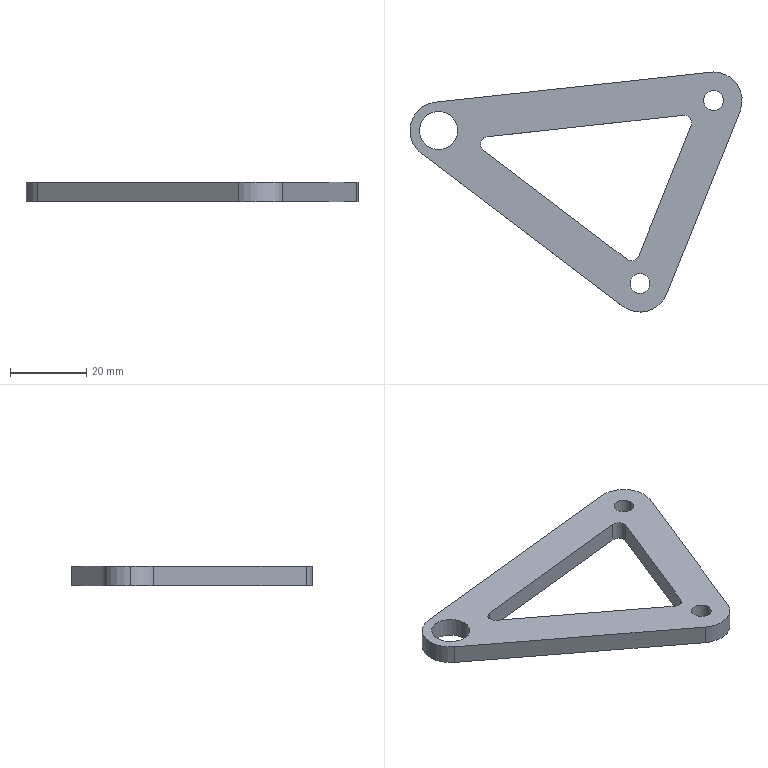Part | SolidWorks | features Extrusion 1 | 1 solid | 22 faces | box 87.181 x 63.036 x 5 mm | volume 10086 mm3 | cylinder 14 | plane 8 | commonest cylinder face diameters 4 x4 5.2 x4 15 x4 10 x2
STEP:
#1=CARTESIAN_POINT('',(-2.6,0.,5.));
#2=VERTEX_POINT('',#1);
#3=CARTESIAN_POINT('',(2.6,0.,5.));
#4=VERTEX_POINT('',#3);
#5=CARTESIAN_POINT('',(0.,0.,5.));
#6=DIRECTION('',(0.,0.,1.));
#7=DIRECTION('',(1.,0.,0.));
#8=AXIS2_PLACEMENT_3D('',#5,#6,#7);
#9=CIRCLE('',#8,2.6);
#10=EDGE_CURVE('',#2,#4,#9,.T.);
#11=ORIENTED_EDGE('',*,*,#10,.T.);
#12=CARTESIAN_POINT('',(2.6,0.,0.));
#13=VERTEX_POINT('',#12);
#14=CARTESIAN_POINT('',(2.6,0.,5.));
#15=DIRECTION('',(0.,0.,-1.));
#16=VECTOR('',#15,1000.);
#17=LINE('',#14,#16);
#18=EDGE_CURVE('',#4,#13,#17,.T.);
#19=ORIENTED_EDGE('',*,*,#18,.T.);
#20=CARTESIAN_POINT('',(-2.6,0.,0.));
#21=VERTEX_POINT('',#20);
#22=CARTESIAN_POINT('',(0.,0.,0.));
#23=DIRECTION('',(0.,0.,1.));
#24=DIRECTION('',(1.,0.,0.));
#25=AXIS2_PLACEMENT_3D('',#22,#23,#24);
#26=CIRCLE('',#25,2.6);
#27=EDGE_CURVE('',#21,#13,#26,.T.);
#28=ORIENTED_EDGE('',*,*,#27,.F.);
#29=CARTESIAN_POINT('',(-2.6,0.,5.));
#30=DIRECTION('',(0.,0.,-1.));
#31=VECTOR('',#30,1000.);
#32=LINE('',#29,#31);
#33=EDGE_CURVE('',#2,#21,#32,.T.);
#34=ORIENTED_EDGE('',*,*,#33,.F.);
#35=EDGE_LOOP('',(#11,#19,#28,#34));
#36=FACE_OUTER_BOUND('',#35,.T.);
#37=CARTESIAN_POINT('',(0.,0.,5.));
#38=DIRECTION('',(0.,0.,-1.));
#39=DIRECTION('',(-1.,0.,0.));
#40=AXIS2_PLACEMENT_3D('',#37,#38,#39);
#41=CYLINDRICAL_SURFACE('',#40,2.6);
#42=ADVANCED_FACE('',(#36),#41,.F.);
#43=CARTESIAN_POINT('',(-77.181,-7.89,5.));
#44=VERTEX_POINT('',#43);
#45=CARTESIAN_POINT('',(-67.181,-7.89,5.));
#46=VERTEX_POINT('',#45);
#47=CARTESIAN_POINT('',(-72.181,-7.89,5.));
#48=DIRECTION('',(0.,0.,1.));
#49=DIRECTION('',(1.,0.,0.));
#50=AXIS2_PLACEMENT_3D('',#47,#48,#49);
#51=CIRCLE('',#50,5.);
#52=EDGE_CURVE('',#44,#46,#51,.T.);
#53=ORIENTED_EDGE('',*,*,#52,.T.);
#54=CARTESIAN_POINT('',(-67.181,-7.89,0.));
#55=VERTEX_POINT('',#54);
#56=CARTESIAN_POINT('',(-67.181,-7.89,5.));
#57=DIRECTION('',(0.,0.,-1.));
#58=VECTOR('',#57,1000.);
#59=LINE('',#56,#58);
#60=EDGE_CURVE('',#46,#55,#59,.T.);
#61=ORIENTED_EDGE('',*,*,#60,.T.);
#62=CARTESIAN_POINT('',(-77.181,-7.89,0.));
#63=VERTEX_POINT('',#62);
#64=CARTESIAN_POINT('',(-72.181,-7.89,0.));
#65=DIRECTION('',(0.,0.,1.));
#66=DIRECTION('',(1.,0.,0.));
#67=AXIS2_PLACEMENT_3D('',#64,#65,#66);
#68=CIRCLE('',#67,5.);
#69=EDGE_CURVE('',#63,#55,#68,.T.);
#70=ORIENTED_EDGE('',*,*,#69,.F.);
#71=CARTESIAN_POINT('',(-77.181,-7.89,5.));
#72=DIRECTION('',(0.,0.,-1.));
#73=VECTOR('',#72,1000.);
#74=LINE('',#71,#73);
#75=EDGE_CURVE('',#44,#63,#74,.T.);
#76=ORIENTED_EDGE('',*,*,#75,.F.);
#77=EDGE_LOOP('',(#53,#61,#70,#76));
#78=FACE_OUTER_BOUND('',#77,.T.);
#79=CARTESIAN_POINT('',(-72.181,-7.89,5.));
#80=DIRECTION('',(0.,0.,-1.));
#81=DIRECTION('',(-1.,0.,0.));
#82=AXIS2_PLACEMENT_3D('',#79,#80,#81);
#83=CYLINDRICAL_SURFACE('',#82,5.);
#84=ADVANCED_FACE('',(#78),#83,.F.);
#85=CARTESIAN_POINT('',(-59.381,-9.509,5.));
#86=VERTEX_POINT('',#85);
#87=CARTESIAN_POINT('',(-61.163,-11.497,5.));
#88=VERTEX_POINT('',#87);
#89=CARTESIAN_POINT('',(-59.163,-11.497,5.));
#90=DIRECTION('',(0.,0.,1.));
#91=DIRECTION('',(-1.,0.,0.));
#92=AXIS2_PLACEMENT_3D('',#89,#90,#91);
#93=CIRCLE('',#92,2.);
#94=EDGE_CURVE('',#86,#88,#93,.T.);
#95=ORIENTED_EDGE('',*,*,#94,.T.);
#96=CARTESIAN_POINT('',(-61.163,-11.497,0.));
#97=VERTEX_POINT('',#96);
#98=CARTESIAN_POINT('',(-61.163,-11.497,5.));
#99=DIRECTION('',(0.,0.,-1.));
#100=VECTOR('',#99,1000.);
#101=LINE('',#98,#100);
#102=EDGE_CURVE('',#88,#97,#101,.T.);
#103=ORIENTED_EDGE('',*,*,#102,.T.);
#104=CARTESIAN_POINT('',(-59.381,-9.509,0.));
#105=VERTEX_POINT('',#104);
#106=CARTESIAN_POINT('',(-59.163,-11.497,0.));
#107=DIRECTION('',(0.,0.,1.));
#108=DIRECTION('',(-1.,0.,0.));
#109=AXIS2_PLACEMENT_3D('',#106,#107,#108);
#110=CIRCLE('',#109,2.);
#111=EDGE_CURVE('',#105,#97,#110,.T.);
#112=ORIENTED_EDGE('',*,*,#111,.F.);
#113=CARTESIAN_POINT('',(-59.381,-9.509,5.));
#114=DIRECTION('',(0.,0.,-1.));
#115=VECTOR('',#114,1000.);
#116=LINE('',#113,#115);
#117=EDGE_CURVE('',#86,#105,#116,.T.);
#118=ORIENTED_EDGE('',*,*,#117,.F.);
#119=EDGE_LOOP('',(#95,#103,#112,#118));
#120=FACE_OUTER_BOUND('',#119,.T.);
#121=CARTESIAN_POINT('',(-59.163,-11.497,5.));
#122=DIRECTION('',(0.,0.,-1.));
#123=DIRECTION('',(-1.,0.,0.));
#124=AXIS2_PLACEMENT_3D('',#121,#122,#123);
#125=CYLINDRICAL_SURFACE('',#124,2.);
#126=ADVANCED_FACE('',(#120),#125,.F.);
#127=CARTESIAN_POINT('',(-21.914,-48.036,5.));
#128=VERTEX_POINT('',#127);
#129=CARTESIAN_POINT('',(-16.714,-48.036,5.));
#130=VERTEX_POINT('',#129);
#131=CARTESIAN_POINT('',(-19.314,-48.036,5.));
#132=DIRECTION('',(0.,0.,1.));
#133=DIRECTION('',(1.,0.,0.));
#134=AXIS2_PLACEMENT_3D('',#131,#132,#133);
#135=CIRCLE('',#134,2.6);
#136=EDGE_CURVE('',#128,#130,#135,.T.);
#137=ORIENTED_EDGE('',*,*,#136,.T.);
#138=CARTESIAN_POINT('',(-16.714,-48.036,0.));
#139=VERTEX_POINT('',#138);
#140=CARTESIAN_POINT('',(-16.714,-48.036,5.));
#141=DIRECTION('',(0.,0.,-1.));
#142=VECTOR('',#141,1000.);
#143=LINE('',#140,#142);
#144=EDGE_CURVE('',#130,#139,#143,.T.);
#145=ORIENTED_EDGE('',*,*,#144,.T.);
#146=CARTESIAN_POINT('',(-21.914,-48.036,0.));
#147=VERTEX_POINT('',#146);
#148=CARTESIAN_POINT('',(-19.314,-48.036,0.));
#149=DIRECTION('',(0.,0.,1.));
#150=DIRECTION('',(1.,0.,0.));
#151=AXIS2_PLACEMENT_3D('',#148,#149,#150);
#152=CIRCLE('',#151,2.6);
#153=EDGE_CURVE('',#147,#139,#152,.T.);
#154=ORIENTED_EDGE('',*,*,#153,.F.);
#155=CARTESIAN_POINT('',(-21.914,-48.036,5.));
#156=DIRECTION('',(0.,0.,-1.));
#157=VECTOR('',#156,1000.);
#158=LINE('',#155,#157);
#159=EDGE_CURVE('',#128,#147,#158,.T.);
#160=ORIENTED_EDGE('',*,*,#159,.F.);
#161=EDGE_LOOP('',(#137,#145,#154,#160));
#162=FACE_OUTER_BOUND('',#161,.T.);
#163=CARTESIAN_POINT('',(-19.314,-48.036,5.));
#164=DIRECTION('',(0.,0.,-1.));
#165=DIRECTION('',(-1.,0.,0.));
#166=AXIS2_PLACEMENT_3D('',#163,#164,#165);
#167=CYLINDRICAL_SURFACE('',#166,2.6);
#168=ADVANCED_FACE('',(#162),#167,.F.);
#169=CARTESIAN_POINT('',(-79.681,-7.89,5.));
#170=VERTEX_POINT('',#169);
#171=CARTESIAN_POINT('',(-76.717,-13.863,5.));
#172=VERTEX_POINT('',#171);
#173=CARTESIAN_POINT('',(-72.181,-7.89,5.));
#174=DIRECTION('',(0.,0.,1.));
#175=DIRECTION('',(1.,0.,0.));
#176=AXIS2_PLACEMENT_3D('',#173,#174,#175);
#177=CIRCLE('',#176,7.5);
#178=EDGE_CURVE('',#170,#172,#177,.T.);
#179=ORIENTED_EDGE('',*,*,#178,.F.);
#180=CARTESIAN_POINT('',(-79.681,-7.89,0.));
#181=VERTEX_POINT('',#180);
#182=CARTESIAN_POINT('',(-79.681,-7.89,5.));
#183=DIRECTION('',(0.,0.,-1.));
#184=VECTOR('',#183,1000.);
#185=LINE('',#182,#184);
#186=EDGE_CURVE('',#170,#181,#185,.T.);
#187=ORIENTED_EDGE('',*,*,#186,.T.);
#188=CARTESIAN_POINT('',(-76.717,-13.863,0.));
#189=VERTEX_POINT('',#188);
#190=CARTESIAN_POINT('',(-72.181,-7.89,0.));
#191=DIRECTION('',(0.,0.,1.));
#192=DIRECTION('',(1.,0.,0.));
#193=AXIS2_PLACEMENT_3D('',#190,#191,#192);
#194=CIRCLE('',#193,7.5);
#195=EDGE_CURVE('',#181,#189,#194,.T.);
#196=ORIENTED_EDGE('',*,*,#195,.T.);
#197=CARTESIAN_POINT('',(-76.717,-13.863,5.));
#198=DIRECTION('',(0.,0.,-1.));
#199=VECTOR('',#198,1000.);
#200=LINE('',#197,#199);
#201=EDGE_CURVE('',#172,#189,#200,.T.);
#202=ORIENTED_EDGE('',*,*,#201,.F.);
#203=EDGE_LOOP('',(#179,#187,#196,#202));
#204=FACE_OUTER_BOUND('',#203,.T.);
#205=CARTESIAN_POINT('',(-72.181,-7.89,5.));
#206=DIRECTION('',(0.,0.,-1.));
#207=DIRECTION('',(-1.,0.,0.));
#208=AXIS2_PLACEMENT_3D('',#205,#206,#207);
#209=CYLINDRICAL_SURFACE('',#208,7.5);
#210=ADVANCED_FACE('',(#204),#209,.T.);
#211=ORIENTED_EDGE('',*,*,#52,.F.);
#212=CARTESIAN_POINT('',(-72.181,-7.89,5.));
#213=DIRECTION('',(0.,0.,1.));
#214=DIRECTION('',(1.,0.,0.));
#215=AXIS2_PLACEMENT_3D('',#212,#213,#214);
#216=CIRCLE('',#215,5.);
#217=EDGE_CURVE('',#46,#44,#216,.T.);
#218=ORIENTED_EDGE('',*,*,#217,.F.);
#219=EDGE_LOOP('',(#211,#218));
#220=FACE_BOUND('',#219,.T.);
#221=CARTESIAN_POINT('',(-72.991,-0.4341,5.));
#222=VERTEX_POINT('',#221);
#223=CARTESIAN_POINT('',(-72.181,-7.89,5.));
#224=DIRECTION('',(0.,0.,1.));
#225=DIRECTION('',(1.,0.,0.));
#226=AXIS2_PLACEMENT_3D('',#223,#224,#225);
#227=CIRCLE('',#226,7.5);
#228=EDGE_CURVE('',#222,#170,#227,.T.);
#229=ORIENTED_EDGE('',*,*,#228,.T.);
#230=ORIENTED_EDGE('',*,*,#178,.T.);
#231=CARTESIAN_POINT('',(-23.849,-54.009,5.));
#232=VERTEX_POINT('',#231);
#233=CARTESIAN_POINT('',(-76.717,-13.863,5.));
#234=DIRECTION('',(0.7964,-0.6048,0.));
#235=VECTOR('',#234,1000.);
#236=LINE('',#233,#235);
#237=EDGE_CURVE('',#172,#232,#236,.T.);
#238=ORIENTED_EDGE('',*,*,#237,.T.);
#239=CARTESIAN_POINT('',(-12.355,-50.834,5.));
#240=VERTEX_POINT('',#239);
#241=CARTESIAN_POINT('',(-19.314,-48.036,5.));
#242=DIRECTION('',(0.,0.,1.));
#243=DIRECTION('',(1.,0.,0.));
#244=AXIS2_PLACEMENT_3D('',#241,#242,#243);
#245=CIRCLE('',#244,7.5);
#246=EDGE_CURVE('',#232,#240,#245,.T.);
#247=ORIENTED_EDGE('',*,*,#246,.T.);
#248=CARTESIAN_POINT('',(6.959,-2.798,5.));
#249=VERTEX_POINT('',#248);
#250=CARTESIAN_POINT('',(6.959,-2.798,5.));
#251=DIRECTION('',(0.373,0.9278,0.));
#252=VECTOR('',#251,1000.);
#253=LINE('',#250,#252);
#254=EDGE_CURVE('',#240,#249,#253,.T.);
#255=ORIENTED_EDGE('',*,*,#254,.T.);
#256=CARTESIAN_POINT('',(0.,7.5,5.));
#257=VERTEX_POINT('',#256);
#258=CARTESIAN_POINT('',(0.,0.,5.));
#259=DIRECTION('',(0.,0.,1.));
#260=DIRECTION('',(1.,0.,0.));
#261=AXIS2_PLACEMENT_3D('',#258,#259,#260);
#262=CIRCLE('',#261,7.5);
#263=EDGE_CURVE('',#249,#257,#262,.T.);
#264=ORIENTED_EDGE('',*,*,#263,.T.);
#265=CARTESIAN_POINT('',(-72.991,-0.4341,5.));
#266=DIRECTION('',(-0.9941,-0.1081,0.));
#267=VECTOR('',#266,1000.);
#268=LINE('',#265,#267);
#269=EDGE_CURVE('',#257,#222,#268,.T.);
#270=ORIENTED_EDGE('',*,*,#269,.T.);
#271=EDGE_LOOP('',(#229,#230,#238,#247,#255,#264,#270));
#272=FACE_OUTER_BOUND('',#271,.T.);
#273=ORIENTED_EDGE('',*,*,#136,.F.);
#274=CARTESIAN_POINT('',(-19.314,-48.036,5.));
#275=DIRECTION('',(0.,0.,1.));
#276=DIRECTION('',(1.,0.,0.));
#277=AXIS2_PLACEMENT_3D('',#274,#275,#276);
#278=CIRCLE('',#277,2.6);
#279=EDGE_CURVE('',#130,#128,#278,.T.);
#280=ORIENTED_EDGE('',*,*,#279,.F.);
#281=EDGE_LOOP('',(#273,#280));
#282=FACE_BOUND('',#281,.T.);
#283=CARTESIAN_POINT('',(-19.653,-40.837,5.));
#284=VERTEX_POINT('',#283);
#285=CARTESIAN_POINT('',(-5.896,-6.623,5.));
#286=VERTEX_POINT('',#285);
#287=CARTESIAN_POINT('',(-19.653,-40.837,5.));
#288=DIRECTION('',(0.373,0.9278,0.));
#289=VECTOR('',#288,1000.);
#290=LINE('',#287,#289);
#291=EDGE_CURVE('',#284,#286,#290,.T.);
#292=ORIENTED_EDGE('',*,*,#291,.F.);
#293=CARTESIAN_POINT('',(-22.718,-41.684,5.));
#294=VERTEX_POINT('',#293);
#295=CARTESIAN_POINT('',(-21.508,-40.091,5.));
#296=DIRECTION('',(0.,0.,1.));
#297=DIRECTION('',(-1.,0.,0.));
#298=AXIS2_PLACEMENT_3D('',#295,#296,#297);
#299=CIRCLE('',#298,2.);
#300=EDGE_CURVE('',#294,#284,#299,.T.);
#301=ORIENTED_EDGE('',*,*,#300,.F.);
#302=CARTESIAN_POINT('',(-60.373,-13.09,5.));
#303=VERTEX_POINT('',#302);
#304=CARTESIAN_POINT('',(-60.373,-13.09,5.));
#305=DIRECTION('',(0.7964,-0.6048,0.));
#306=VECTOR('',#305,1000.);
#307=LINE('',#304,#306);
#308=EDGE_CURVE('',#303,#294,#307,.T.);
#309=ORIENTED_EDGE('',*,*,#308,.F.);
#310=CARTESIAN_POINT('',(-59.163,-11.497,5.));
#311=DIRECTION('',(0.,0.,1.));
#312=DIRECTION('',(-1.,0.,0.));
#313=AXIS2_PLACEMENT_3D('',#310,#311,#312);
#314=CIRCLE('',#313,2.);
#315=EDGE_CURVE('',#88,#303,#314,.T.);
#316=ORIENTED_EDGE('',*,*,#315,.F.);
#317=ORIENTED_EDGE('',*,*,#94,.F.);
#318=CARTESIAN_POINT('',(-7.969,-3.889,5.));
#319=VERTEX_POINT('',#318);
#320=CARTESIAN_POINT('',(-7.969,-3.889,5.));
#321=DIRECTION('',(-0.9941,-0.1087,0.));
#322=VECTOR('',#321,1000.);
#323=LINE('',#320,#322);
#324=EDGE_CURVE('',#319,#86,#323,.T.);
#325=ORIENTED_EDGE('',*,*,#324,.F.);
#326=CARTESIAN_POINT('',(-7.752,-5.877,5.));
#327=DIRECTION('',(0.,0.,1.));
#328=DIRECTION('',(1.,0.,0.));
#329=AXIS2_PLACEMENT_3D('',#326,#327,#328);
#330=CIRCLE('',#329,2.);
#331=EDGE_CURVE('',#286,#319,#330,.T.);
#332=ORIENTED_EDGE('',*,*,#331,.F.);
#333=EDGE_LOOP('',(#292,#301,#309,#316,#317,#325,#332));
#334=FACE_BOUND('',#333,.T.);
#335=ORIENTED_EDGE('',*,*,#10,.F.);
#336=CARTESIAN_POINT('',(0.,0.,5.));
#337=DIRECTION('',(0.,0.,1.));
#338=DIRECTION('',(1.,0.,0.));
#339=AXIS2_PLACEMENT_3D('',#336,#337,#338);
#340=CIRCLE('',#339,2.6);
#341=EDGE_CURVE('',#4,#2,#340,.T.);
#342=ORIENTED_EDGE('',*,*,#341,.F.);
#343=EDGE_LOOP('',(#335,#342));
#344=FACE_BOUND('',#343,.T.);
#345=CARTESIAN_POINT('',(-72.181,-7.89,5.));
#346=DIRECTION('',(0.,0.,1.));
#347=DIRECTION('',(1.,0.,0.));
#348=AXIS2_PLACEMENT_3D('',#345,#346,#347);
#349=PLANE('',#348);
#350=ADVANCED_FACE('',(#220,#272,#282,#334,#344),#349,.T.);
#351=ORIENTED_EDGE('',*,*,#153,.T.);
#352=CARTESIAN_POINT('',(-19.314,-48.036,0.));
#353=DIRECTION('',(0.,0.,1.));
#354=DIRECTION('',(1.,0.,0.));
#355=AXIS2_PLACEMENT_3D('',#352,#353,#354);
#356=CIRCLE('',#355,2.6);
#357=EDGE_CURVE('',#139,#147,#356,.T.);
#358=ORIENTED_EDGE('',*,*,#357,.T.);
#359=EDGE_LOOP('',(#351,#358));
#360=FACE_BOUND('',#359,.T.);
#361=CARTESIAN_POINT('',(-72.991,-0.4341,0.));
#362=VERTEX_POINT('',#361);
#363=CARTESIAN_POINT('',(-72.181,-7.89,0.));
#364=DIRECTION('',(0.,0.,1.));
#365=DIRECTION('',(1.,0.,0.));
#366=AXIS2_PLACEMENT_3D('',#363,#364,#365);
#367=CIRCLE('',#366,7.5);
#368=EDGE_CURVE('',#362,#181,#367,.T.);
#369=ORIENTED_EDGE('',*,*,#368,.F.);
#370=CARTESIAN_POINT('',(0.,7.5,0.));
#371=VERTEX_POINT('',#370);
#372=CARTESIAN_POINT('',(-72.991,-0.4341,0.));
#373=DIRECTION('',(-0.9941,-0.1081,0.));
#374=VECTOR('',#373,1000.);
#375=LINE('',#372,#374);
#376=EDGE_CURVE('',#371,#362,#375,.T.);
#377=ORIENTED_EDGE('',*,*,#376,.F.);
#378=CARTESIAN_POINT('',(6.959,-2.798,0.));
#379=VERTEX_POINT('',#378);
#380=CARTESIAN_POINT('',(0.,0.,0.));
#381=DIRECTION('',(0.,0.,1.));
#382=DIRECTION('',(1.,0.,0.));
#383=AXIS2_PLACEMENT_3D('',#380,#381,#382);
#384=CIRCLE('',#383,7.5);
#385=EDGE_CURVE('',#379,#371,#384,.T.);
#386=ORIENTED_EDGE('',*,*,#385,.F.);
#387=CARTESIAN_POINT('',(-12.355,-50.834,0.));
#388=VERTEX_POINT('',#387);
#389=CARTESIAN_POINT('',(6.959,-2.798,0.));
#390=DIRECTION('',(0.373,0.9278,0.));
#391=VECTOR('',#390,1000.);
#392=LINE('',#389,#391);
#393=EDGE_CURVE('',#388,#379,#392,.T.);
#394=ORIENTED_EDGE('',*,*,#393,.F.);
#395=CARTESIAN_POINT('',(-23.849,-54.009,0.));
#396=VERTEX_POINT('',#395);
#397=CARTESIAN_POINT('',(-19.314,-48.036,0.));
#398=DIRECTION('',(0.,0.,1.));
#399=DIRECTION('',(1.,0.,0.));
#400=AXIS2_PLACEMENT_3D('',#397,#398,#399);
#401=CIRCLE('',#400,7.5);
#402=EDGE_CURVE('',#396,#388,#401,.T.);
#403=ORIENTED_EDGE('',*,*,#402,.F.);
#404=CARTESIAN_POINT('',(-76.717,-13.863,0.));
#405=DIRECTION('',(0.7964,-0.6048,0.));
#406=VECTOR('',#405,1000.);
#407=LINE('',#404,#406);
#408=EDGE_CURVE('',#189,#396,#407,.T.);
#409=ORIENTED_EDGE('',*,*,#408,.F.);
#410=ORIENTED_EDGE('',*,*,#195,.F.);
#411=EDGE_LOOP('',(#369,#377,#386,#394,#403,#409,#410));
#412=FACE_OUTER_BOUND('',#411,.T.);
#413=CARTESIAN_POINT('',(-22.718,-41.684,0.));
#414=VERTEX_POINT('',#413);
#415=CARTESIAN_POINT('',(-19.653,-40.837,0.));
#416=VERTEX_POINT('',#415);
#417=CARTESIAN_POINT('',(-21.508,-40.091,0.));
#418=DIRECTION('',(0.,0.,1.));
#419=DIRECTION('',(-1.,0.,0.));
#420=AXIS2_PLACEMENT_3D('',#417,#418,#419);
#421=CIRCLE('',#420,2.);
#422=EDGE_CURVE('',#414,#416,#421,.T.);
#423=ORIENTED_EDGE('',*,*,#422,.T.);
#424=CARTESIAN_POINT('',(-5.896,-6.623,0.));
#425=VERTEX_POINT('',#424);
#426=CARTESIAN_POINT('',(-19.653,-40.837,0.));
#427=DIRECTION('',(0.373,0.9278,0.));
#428=VECTOR('',#427,1000.);
#429=LINE('',#426,#428);
#430=EDGE_CURVE('',#416,#425,#429,.T.);
#431=ORIENTED_EDGE('',*,*,#430,.T.);
#432=CARTESIAN_POINT('',(-7.969,-3.889,0.));
#433=VERTEX_POINT('',#432);
#434=CARTESIAN_POINT('',(-7.752,-5.877,0.));
#435=DIRECTION('',(0.,0.,1.));
#436=DIRECTION('',(1.,0.,0.));
#437=AXIS2_PLACEMENT_3D('',#434,#435,#436);
#438=CIRCLE('',#437,2.);
#439=EDGE_CURVE('',#425,#433,#438,.T.);
#440=ORIENTED_EDGE('',*,*,#439,.T.);
#441=CARTESIAN_POINT('',(-7.969,-3.889,0.));
#442=DIRECTION('',(-0.9941,-0.1087,0.));
#443=VECTOR('',#442,1000.);
#444=LINE('',#441,#443);
#445=EDGE_CURVE('',#433,#105,#444,.T.);
#446=ORIENTED_EDGE('',*,*,#445,.T.);
#447=ORIENTED_EDGE('',*,*,#111,.T.);
#448=CARTESIAN_POINT('',(-60.373,-13.09,0.));
#449=VERTEX_POINT('',#448);
#450=CARTESIAN_POINT('',(-59.163,-11.497,0.));
#451=DIRECTION('',(0.,0.,1.));
#452=DIRECTION('',(-1.,0.,0.));
#453=AXIS2_PLACEMENT_3D('',#450,#451,#452);
#454=CIRCLE('',#453,2.);
#455=EDGE_CURVE('',#97,#449,#454,.T.);
#456=ORIENTED_EDGE('',*,*,#455,.T.);
#457=CARTESIAN_POINT('',(-60.373,-13.09,0.));
#458=DIRECTION('',(0.7964,-0.6048,0.));
#459=VECTOR('',#458,1000.);
#460=LINE('',#457,#459);
#461=EDGE_CURVE('',#449,#414,#460,.T.);
#462=ORIENTED_EDGE('',*,*,#461,.T.);
#463=EDGE_LOOP('',(#423,#431,#440,#446,#447,#456,#462));
#464=FACE_BOUND('',#463,.T.);
#465=ORIENTED_EDGE('',*,*,#69,.T.);
#466=CARTESIAN_POINT('',(-72.181,-7.89,0.));
#467=DIRECTION('',(0.,0.,1.));
#468=DIRECTION('',(1.,0.,0.));
#469=AXIS2_PLACEMENT_3D('',#466,#467,#468);
#470=CIRCLE('',#469,5.);
#471=EDGE_CURVE('',#55,#63,#470,.T.);
#472=ORIENTED_EDGE('',*,*,#471,.T.);
#473=EDGE_LOOP('',(#465,#472));
#474=FACE_BOUND('',#473,.T.);
#475=ORIENTED_EDGE('',*,*,#27,.T.);
#476=CARTESIAN_POINT('',(0.,0.,0.));
#477=DIRECTION('',(0.,0.,1.));
#478=DIRECTION('',(1.,0.,0.));
#479=AXIS2_PLACEMENT_3D('',#476,#477,#478);
#480=CIRCLE('',#479,2.6);
#481=EDGE_CURVE('',#13,#21,#480,.T.);
#482=ORIENTED_EDGE('',*,*,#481,.T.);
#483=EDGE_LOOP('',(#475,#482));
#484=FACE_BOUND('',#483,.T.);
#485=CARTESIAN_POINT('',(-72.181,-7.89,0.));
#486=DIRECTION('',(0.,0.,1.));
#487=DIRECTION('',(1.,0.,0.));
#488=AXIS2_PLACEMENT_3D('',#485,#486,#487);
#489=PLANE('',#488);
#490=ADVANCED_FACE('',(#360,#412,#464,#474,#484),#489,.F.);
#491=ORIENTED_EDGE('',*,*,#186,.F.);
#492=ORIENTED_EDGE('',*,*,#228,.F.);
#493=CARTESIAN_POINT('',(-72.991,-0.4341,5.));
#494=DIRECTION('',(0.,0.,-1.));
#495=VECTOR('',#494,1000.);
#496=LINE('',#493,#495);
#497=EDGE_CURVE('',#222,#362,#496,.T.);
#498=ORIENTED_EDGE('',*,*,#497,.T.);
#499=ORIENTED_EDGE('',*,*,#368,.T.);
#500=EDGE_LOOP('',(#491,#492,#498,#499));
#501=FACE_OUTER_BOUND('',#500,.T.);
#502=CARTESIAN_POINT('',(-72.181,-7.89,5.));
#503=DIRECTION('',(0.,0.,-1.));
#504=DIRECTION('',(-1.,0.,0.));
#505=AXIS2_PLACEMENT_3D('',#502,#503,#504);
#506=CYLINDRICAL_SURFACE('',#505,7.5);
#507=ADVANCED_FACE('',(#501),#506,.T.);
#508=ORIENTED_EDGE('',*,*,#408,.T.);
#509=CARTESIAN_POINT('',(-23.849,-54.009,5.));
#510=DIRECTION('',(0.,0.,-1.));
#511=VECTOR('',#510,1000.);
#512=LINE('',#509,#511);
#513=EDGE_CURVE('',#232,#396,#512,.T.);
#514=ORIENTED_EDGE('',*,*,#513,.F.);
#515=ORIENTED_EDGE('',*,*,#237,.F.);
#516=ORIENTED_EDGE('',*,*,#201,.T.);
#517=EDGE_LOOP('',(#508,#514,#515,#516));
#518=FACE_OUTER_BOUND('',#517,.T.);
#519=CARTESIAN_POINT('',(-76.717,-13.863,5.));
#520=DIRECTION('',(0.6048,0.7964,0.));
#521=DIRECTION('',(-0.7964,0.6048,0.));
#522=AXIS2_PLACEMENT_3D('',#519,#520,#521);
#523=PLANE('',#522);
#524=ADVANCED_FACE('',(#518),#523,.F.);
#525=ORIENTED_EDGE('',*,*,#402,.T.);
#526=CARTESIAN_POINT('',(-12.355,-50.834,5.));
#527=DIRECTION('',(0.,0.,-1.));
#528=VECTOR('',#527,1000.);
#529=LINE('',#526,#528);
#530=EDGE_CURVE('',#240,#388,#529,.T.);
#531=ORIENTED_EDGE('',*,*,#530,.F.);
#532=ORIENTED_EDGE('',*,*,#246,.F.);
#533=ORIENTED_EDGE('',*,*,#513,.T.);
#534=EDGE_LOOP('',(#525,#531,#532,#533));
#535=FACE_OUTER_BOUND('',#534,.T.);
#536=CARTESIAN_POINT('',(-19.314,-48.036,5.));
#537=DIRECTION('',(0.,0.,-1.));
#538=DIRECTION('',(-1.,0.,0.));
#539=AXIS2_PLACEMENT_3D('',#536,#537,#538);
#540=CYLINDRICAL_SURFACE('',#539,7.5);
#541=ADVANCED_FACE('',(#535),#540,.T.);
#542=ORIENTED_EDGE('',*,*,#393,.T.);
#543=CARTESIAN_POINT('',(6.959,-2.798,5.));
#544=DIRECTION('',(0.,0.,-1.));
#545=VECTOR('',#544,1000.);
#546=LINE('',#543,#545);
#547=EDGE_CURVE('',#249,#379,#546,.T.);
#548=ORIENTED_EDGE('',*,*,#547,.F.);
#549=ORIENTED_EDGE('',*,*,#254,.F.);
#550=ORIENTED_EDGE('',*,*,#530,.T.);
#551=EDGE_LOOP('',(#542,#548,#549,#550));
#552=FACE_OUTER_BOUND('',#551,.T.);
#553=CARTESIAN_POINT('',(6.959,-2.798,5.));
#554=DIRECTION('',(-0.9278,0.373,0.));
#555=DIRECTION('',(-0.373,-0.9278,0.));
#556=AXIS2_PLACEMENT_3D('',#553,#554,#555);
#557=PLANE('',#556);
#558=ADVANCED_FACE('',(#552),#557,.F.);
#559=ORIENTED_EDGE('',*,*,#385,.T.);
#560=CARTESIAN_POINT('',(0.,7.5,5.));
#561=DIRECTION('',(0.,0.,-1.));
#562=VECTOR('',#561,1000.);
#563=LINE('',#560,#562);
#564=EDGE_CURVE('',#257,#371,#563,.T.);
#565=ORIENTED_EDGE('',*,*,#564,.F.);
#566=ORIENTED_EDGE('',*,*,#263,.F.);
#567=ORIENTED_EDGE('',*,*,#547,.T.);
#568=EDGE_LOOP('',(#559,#565,#566,#567));
#569=FACE_OUTER_BOUND('',#568,.T.);
#570=CARTESIAN_POINT('',(0.,0.,5.));
#571=DIRECTION('',(0.,0.,-1.));
#572=DIRECTION('',(-1.,0.,0.));
#573=AXIS2_PLACEMENT_3D('',#570,#571,#572);
#574=CYLINDRICAL_SURFACE('',#573,7.5);
#575=ADVANCED_FACE('',(#569),#574,.T.);
#576=ORIENTED_EDGE('',*,*,#376,.T.);
#577=ORIENTED_EDGE('',*,*,#497,.F.);
#578=ORIENTED_EDGE('',*,*,#269,.F.);
#579=ORIENTED_EDGE('',*,*,#564,.T.);
#580=EDGE_LOOP('',(#576,#577,#578,#579));
#581=FACE_OUTER_BOUND('',#580,.T.);
#582=CARTESIAN_POINT('',(-72.991,-0.4341,5.));
#583=DIRECTION('',(0.1081,-0.9941,0.));
#584=DIRECTION('',(0.9941,0.1081,0.));
#585=AXIS2_PLACEMENT_3D('',#582,#583,#584);
#586=PLANE('',#585);
#587=ADVANCED_FACE('',(#581),#586,.F.);
#588=ORIENTED_EDGE('',*,*,#144,.F.);
#589=ORIENTED_EDGE('',*,*,#279,.T.);
#590=ORIENTED_EDGE('',*,*,#159,.T.);
#591=ORIENTED_EDGE('',*,*,#357,.F.);
#592=EDGE_LOOP('',(#588,#589,#590,#591));
#593=FACE_OUTER_BOUND('',#592,.T.);
#594=CARTESIAN_POINT('',(-19.314,-48.036,5.));
#595=DIRECTION('',(0.,0.,-1.));
#596=DIRECTION('',(-1.,0.,0.));
#597=AXIS2_PLACEMENT_3D('',#594,#595,#596);
#598=CYLINDRICAL_SURFACE('',#597,2.6);
#599=ADVANCED_FACE('',(#593),#598,.F.);
#600=ORIENTED_EDGE('',*,*,#422,.F.);
#601=CARTESIAN_POINT('',(-22.718,-41.684,5.));
#602=DIRECTION('',(0.,0.,-1.));
#603=VECTOR('',#602,1000.);
#604=LINE('',#601,#603);
#605=EDGE_CURVE('',#294,#414,#604,.T.);
#606=ORIENTED_EDGE('',*,*,#605,.F.);
#607=ORIENTED_EDGE('',*,*,#300,.T.);
#608=CARTESIAN_POINT('',(-19.653,-40.837,5.));
#609=DIRECTION('',(0.,0.,-1.));
#610=VECTOR('',#609,1000.);
#611=LINE('',#608,#610);
#612=EDGE_CURVE('',#284,#416,#611,.T.);
#613=ORIENTED_EDGE('',*,*,#612,.T.);
#614=EDGE_LOOP('',(#600,#606,#607,#613));
#615=FACE_OUTER_BOUND('',#614,.T.);
#616=CARTESIAN_POINT('',(-21.508,-40.091,5.));
#617=DIRECTION('',(0.,0.,-1.));
#618=DIRECTION('',(-1.,0.,0.));
#619=AXIS2_PLACEMENT_3D('',#616,#617,#618);
#620=CYLINDRICAL_SURFACE('',#619,2.);
#621=ADVANCED_FACE('',(#615),#620,.F.);
#622=ORIENTED_EDGE('',*,*,#430,.F.);
#623=ORIENTED_EDGE('',*,*,#612,.F.);
#624=ORIENTED_EDGE('',*,*,#291,.T.);
#625=CARTESIAN_POINT('',(-5.896,-6.623,5.));
#626=DIRECTION('',(0.,0.,-1.));
#627=VECTOR('',#626,1000.);
#628=LINE('',#625,#627);
#629=EDGE_CURVE('',#286,#425,#628,.T.);
#630=ORIENTED_EDGE('',*,*,#629,.T.);
#631=EDGE_LOOP('',(#622,#623,#624,#630));
#632=FACE_OUTER_BOUND('',#631,.T.);
#633=CARTESIAN_POINT('',(-19.653,-40.837,5.));
#634=DIRECTION('',(-0.9278,0.373,0.));
#635=DIRECTION('',(-0.373,-0.9278,0.));
#636=AXIS2_PLACEMENT_3D('',#633,#634,#635);
#637=PLANE('',#636);
#638=ADVANCED_FACE('',(#632),#637,.T.);
#639=ORIENTED_EDGE('',*,*,#439,.F.);
#640=ORIENTED_EDGE('',*,*,#629,.F.);
#641=ORIENTED_EDGE('',*,*,#331,.T.);
#642=CARTESIAN_POINT('',(-7.969,-3.889,5.));
#643=DIRECTION('',(0.,0.,-1.));
#644=VECTOR('',#643,1000.);
#645=LINE('',#642,#644);
#646=EDGE_CURVE('',#319,#433,#645,.T.);
#647=ORIENTED_EDGE('',*,*,#646,.T.);
#648=EDGE_LOOP('',(#639,#640,#641,#647));
#649=FACE_OUTER_BOUND('',#648,.T.);
#650=CARTESIAN_POINT('',(-7.752,-5.877,5.));
#651=DIRECTION('',(0.,0.,-1.));
#652=DIRECTION('',(-1.,0.,0.));
#653=AXIS2_PLACEMENT_3D('',#650,#651,#652);
#654=CYLINDRICAL_SURFACE('',#653,2.);
#655=ADVANCED_FACE('',(#649),#654,.F.);
#656=ORIENTED_EDGE('',*,*,#445,.F.);
#657=ORIENTED_EDGE('',*,*,#646,.F.);
#658=ORIENTED_EDGE('',*,*,#324,.T.);
#659=ORIENTED_EDGE('',*,*,#117,.T.);
#660=EDGE_LOOP('',(#656,#657,#658,#659));
#661=FACE_OUTER_BOUND('',#660,.T.);
#662=CARTESIAN_POINT('',(-7.969,-3.889,5.));
#663=DIRECTION('',(0.1087,-0.9941,0.));
#664=DIRECTION('',(0.9941,0.1087,0.));
#665=AXIS2_PLACEMENT_3D('',#662,#663,#664);
#666=PLANE('',#665);
#667=ADVANCED_FACE('',(#661),#666,.T.);
#668=ORIENTED_EDGE('',*,*,#102,.F.);
#669=ORIENTED_EDGE('',*,*,#315,.T.);
#670=CARTESIAN_POINT('',(-60.373,-13.09,5.));
#671=DIRECTION('',(0.,0.,-1.));
#672=VECTOR('',#671,1000.);
#673=LINE('',#670,#672);
#674=EDGE_CURVE('',#303,#449,#673,.T.);
#675=ORIENTED_EDGE('',*,*,#674,.T.);
#676=ORIENTED_EDGE('',*,*,#455,.F.);
#677=EDGE_LOOP('',(#668,#669,#675,#676));
#678=FACE_OUTER_BOUND('',#677,.T.);
#679=CARTESIAN_POINT('',(-59.163,-11.497,5.));
#680=DIRECTION('',(0.,0.,-1.));
#681=DIRECTION('',(-1.,0.,0.));
#682=AXIS2_PLACEMENT_3D('',#679,#680,#681);
#683=CYLINDRICAL_SURFACE('',#682,2.);
#684=ADVANCED_FACE('',(#678),#683,.F.);
#685=ORIENTED_EDGE('',*,*,#461,.F.);
#686=ORIENTED_EDGE('',*,*,#674,.F.);
#687=ORIENTED_EDGE('',*,*,#308,.T.);
#688=ORIENTED_EDGE('',*,*,#605,.T.);
#689=EDGE_LOOP('',(#685,#686,#687,#688));
#690=FACE_OUTER_BOUND('',#689,.T.);
#691=CARTESIAN_POINT('',(-60.373,-13.09,5.));
#692=DIRECTION('',(0.6048,0.7964,0.));
#693=DIRECTION('',(-0.7964,0.6048,0.));
#694=AXIS2_PLACEMENT_3D('',#691,#692,#693);
#695=PLANE('',#694);
#696=ADVANCED_FACE('',(#690),#695,.T.);
#697=ORIENTED_EDGE('',*,*,#60,.F.);
#698=ORIENTED_EDGE('',*,*,#217,.T.);
#699=ORIENTED_EDGE('',*,*,#75,.T.);
#700=ORIENTED_EDGE('',*,*,#471,.F.);
#701=EDGE_LOOP('',(#697,#698,#699,#700));
#702=FACE_OUTER_BOUND('',#701,.T.);
#703=CARTESIAN_POINT('',(-72.181,-7.89,5.));
#704=DIRECTION('',(0.,0.,-1.));
#705=DIRECTION('',(-1.,0.,0.));
#706=AXIS2_PLACEMENT_3D('',#703,#704,#705);
#707=CYLINDRICAL_SURFACE('',#706,5.);
#708=ADVANCED_FACE('',(#702),#707,.F.);
#709=ORIENTED_EDGE('',*,*,#18,.F.);
#710=ORIENTED_EDGE('',*,*,#341,.T.);
#711=ORIENTED_EDGE('',*,*,#33,.T.);
#712=ORIENTED_EDGE('',*,*,#481,.F.);
#713=EDGE_LOOP('',(#709,#710,#711,#712));
#714=FACE_OUTER_BOUND('',#713,.T.);
#715=CARTESIAN_POINT('',(0.,0.,5.));
#716=DIRECTION('',(0.,0.,-1.));
#717=DIRECTION('',(-1.,0.,0.));
#718=AXIS2_PLACEMENT_3D('',#715,#716,#717);
#719=CYLINDRICAL_SURFACE('',#718,2.6);
#720=ADVANCED_FACE('',(#714),#719,.F.);
#721=CLOSED_SHELL('',(#42,#84,#126,#168,#210,#350,#490,#507,#524,#541,#558,#575,#587,#599,#621,#638,#655,#667,#684,#696,#708,#720));
#722=MANIFOLD_SOLID_BREP('',#721);
#723=CARTESIAN_POINT('',(0.,0.,0.));
#724=DIRECTION('',(0.,0.,1.));
#725=DIRECTION('',(1.,0.,0.));
#726=AXIS2_PLACEMENT_3D('',#723,#724,#725);
#727=(LENGTH_UNIT()NAMED_UNIT(*)SI_UNIT(.MILLI.,.METRE.));
#728=UNCERTAINTY_MEASURE_WITH_UNIT(LENGTH_MEASURE(0.00001),#727,'','');
#729=(NAMED_UNIT(*)PLANE_ANGLE_UNIT()SI_UNIT($,.RADIAN.));
#730=(NAMED_UNIT(*)SI_UNIT($,.STERADIAN.)SOLID_ANGLE_UNIT());
#731=(GEOMETRIC_REPRESENTATION_CONTEXT(3)GLOBAL_UNCERTAINTY_ASSIGNED_CONTEXT((#728))GLOBAL_UNIT_ASSIGNED_CONTEXT((#727,#729,#730))REPRESENTATION_CONTEXT('',''));
#732=ADVANCED_BREP_SHAPE_REPRESENTATION('',(#722,#726),#731);